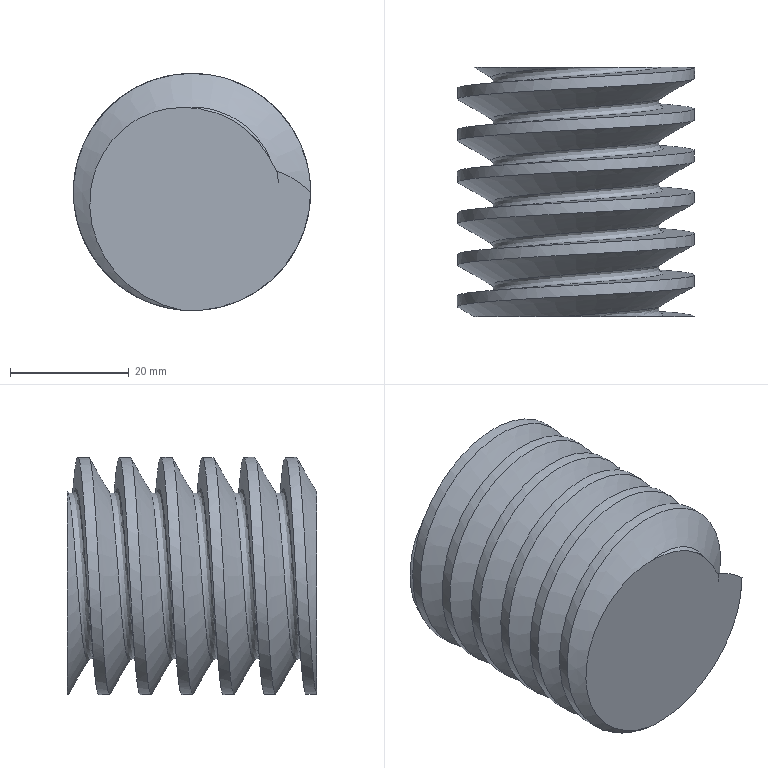Part | NX | features DATUM_CSYS 2, CYLINDER 1, HELIX 1, SKETCH 1, SKIN 1, SUBTRACT 1 | 1 solid | 6 faces | box 40 x 42 x 40 mm | volume 39845 mm3 | spline 3 | plane 2 | cylinder 1 | commonest cylinder face diameters 40 x1